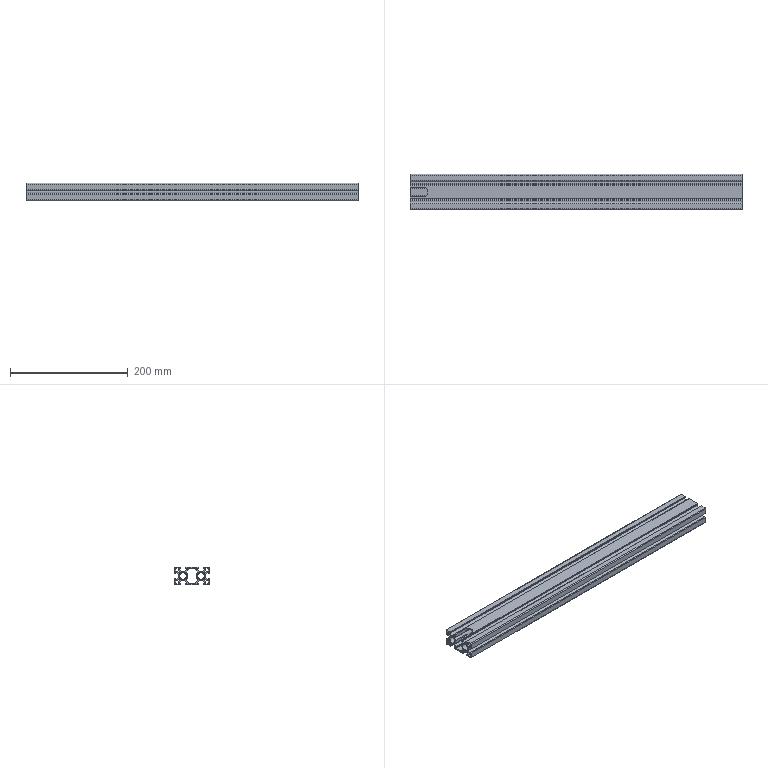Part | STEP file | belt line support ET profile 565 | 1 solid | 165 faces | box 565 x 60 x 30 mm | volume 364592 mm3 | plane 87 | cylinder 70 | cone 8 | commonest cylinder face diameters 2 x26 16 x14 1 x10 12 x8 3 x4 10 x4